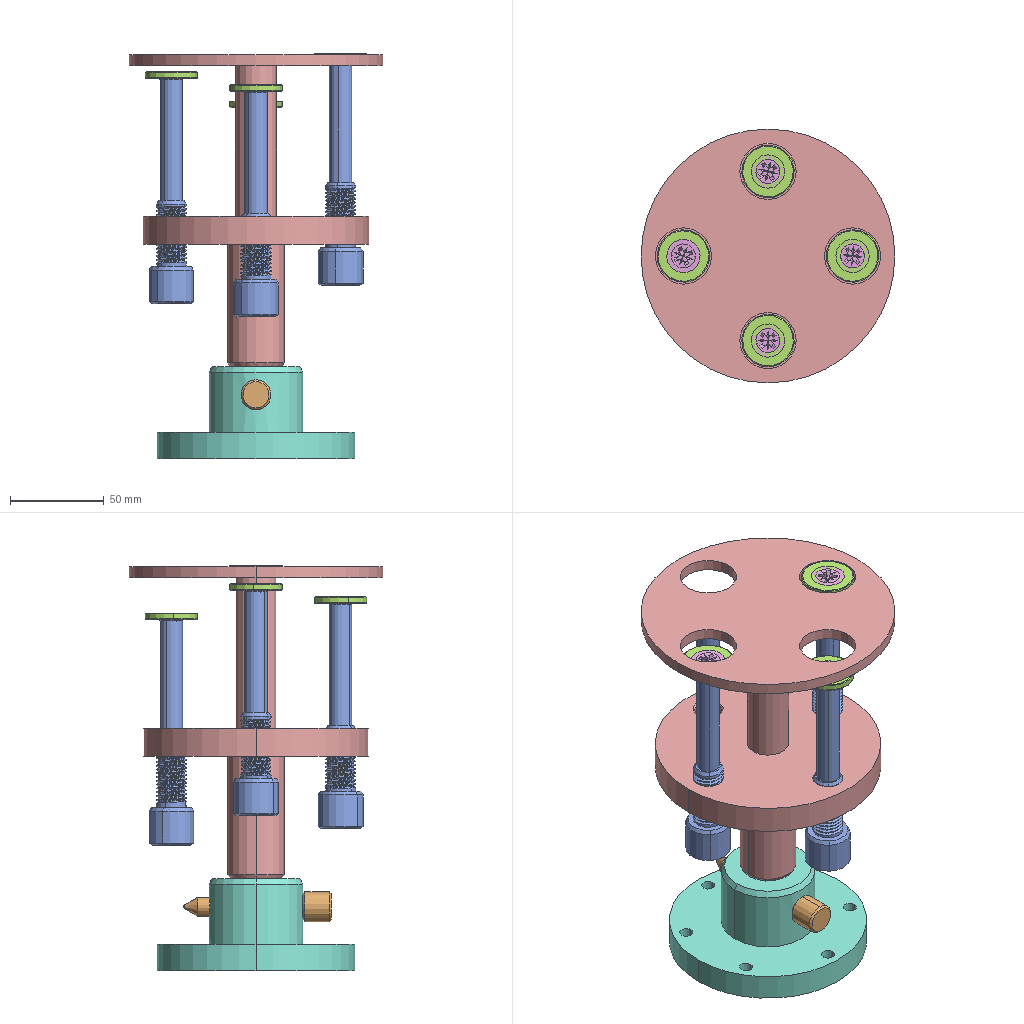Assembly | SolidWorks | 6 different items | 12 placed | box 135 x 135 x 216 mm
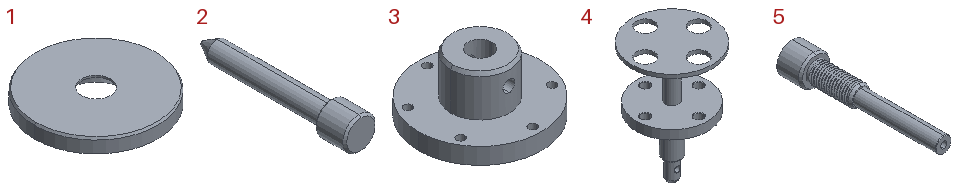Parts list (item | name | quantity | size | volume | features):
1 | - | x4 | 28 x 28 x 3.5 mm | 1892 mm3 | features 3DProfileFeature 1, Chamfer 1, Extrusion 1, HoleWzd 1
2 | - | x1 | 16 x 78.492 x 16 mm | 7592 mm3 | features Chamfer 1, Revolution 1
3 | - | x1 | 105 x 105 x 49 mm | 172934 mm3 | features ICE 2, Chamfer 1, Extrusion 1
4 | - | x1 | 135 x 135 x 201 mm | 313916 mm3 | features ICE 7, Chamfer 2, 3DProfileFeature 1, CirPattern 1, Extrusion 1, HoleWzd 1
5 | - | x4 | 24 x 120 x 24 mm | 22039 mm3 | features Chamfer 2, 3DProfileFeature 1, HoleWzd 1, Revolution 1, SweepThread 1
6 | cross recessed countersunk head screws gb1 | x1 | - | - | -
Mates (type | each side: item.copy, entity, surface, feature):
Concentric | 4.1 face cylinder M16x1.5 Tapped Hole1 | 5.1 face cylinder Revolve1
Concentric | 4.1 face cylinder CirPattern1 | 5.2 face cylinder Revolve1
Concentric | 4.1 face cylinder CirPattern1 | 5.3 face cylinder Revolve1
Concentric | 4.1 face cylinder CirPattern1 | 5.4 face cylinder Revolve1
Coincident | 5.4 face plane Revolve1 | 1.1 face plane Boss-Extrude1
Concentric | 5.4 face cylinder Revolve1 | 1.1 face cylinder Boss-Extrude1
Coincident | 5.1 face plane Revolve1 | 1.2 face plane Boss-Extrude1
Concentric | 5.1 face cylinder Revolve1 | 1.2 face cylinder Boss-Extrude1
Coincident | 5.2 face plane Revolve1 | 1.3 face plane Boss-Extrude1
Concentric | 5.2 face cylinder Revolve1 | 1.3 face cylinder Boss-Extrude1
Coincident | 5.3 face plane Revolve1 | 1.4 face plane Boss-Extrude1
Concentric | 5.3 face cylinder Revolve1 | 1.4 face cylinder Boss-Extrude1
Concentric | 4.1 face cylinder Cut-Extrude2 | 3.1 face cylinder Cut-Extrude1
Concentric | 4.1 face cylinder Boss-Extrude4 | 3.1 face cylinder Boss-Extrude2
Concentric | 3.1 face cylinder Cut-Extrude1 | 2.1 face cylinder Revolve1
Tangent | 3.1 face cylinder Boss-Extrude2 | 2.1 face plane Revolve1